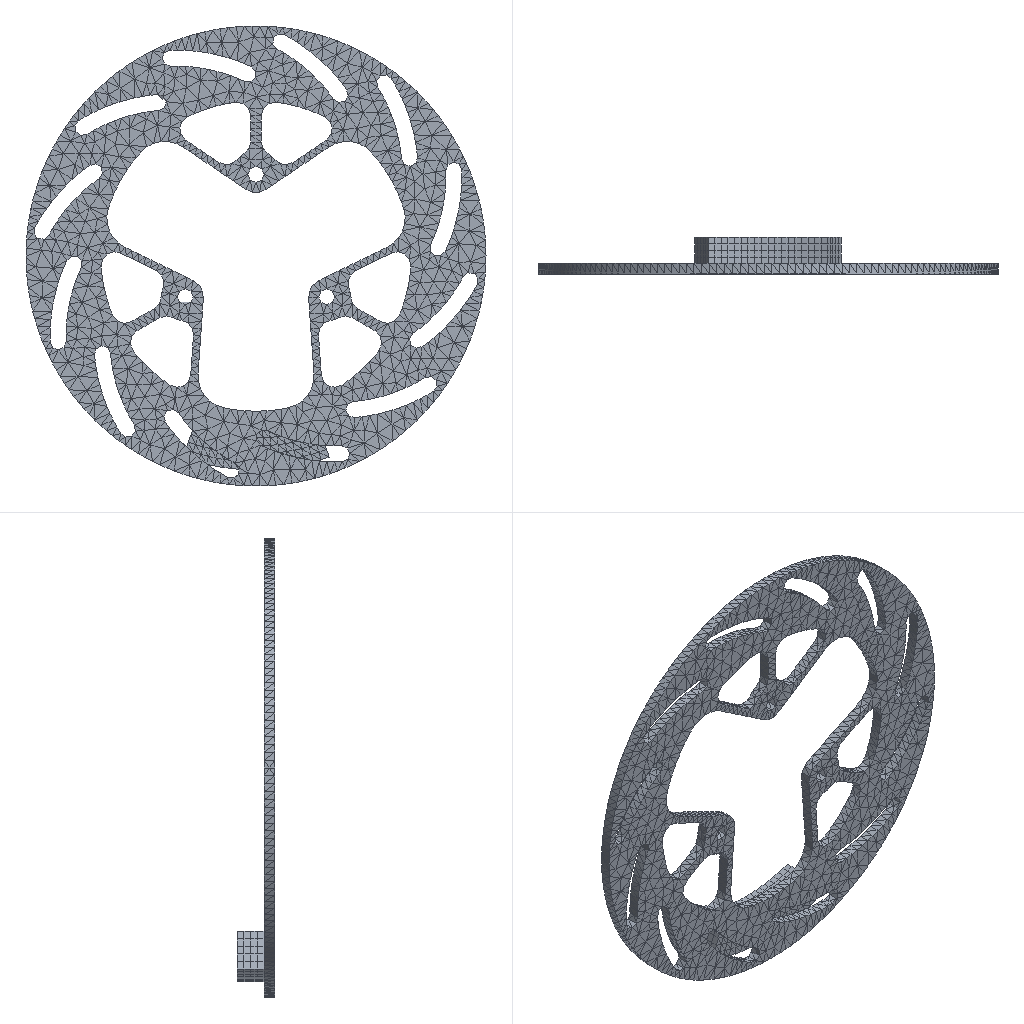Simulation study | ansys workbench
Set-up summary:
category,name,step,type,value,unit,region
solver,ansys_workbench
units,mm-N-s-tonne (MPa),,stated,"/units,MPA"
analysis,LS1,,transient thermal
load_step,LS1,LS1,transient thermal,nsubst=100; time=5
mesh,nodes,,,16602
mesh,elements,,,11231
element_type,SOLID291,,,6582
element_type,SURF152,,,3759
element_type,SOLID279,,,360
element_type,TARGE170,,,265
element_type,CONTA174,,,265
material,HT250,,E,120000,tonne s^-2 mm^-1
material,HT250,,nu,0.26
material,HT250,,density,7.2e-09,tonne mm^-3
material,HT250,,conductivity,44.3,tonne mm s^-3 C^-1
material,HT250,,specific_heat,4.5e+08,mm^2 s^-2 C^-1
material,HT250,,cte,6e-06,C^-1
load,Define Uniform Initial temperature,model,body load temp,22,,all
load,"Create ""?""",LS1,heat flux,1800,,SURF152 #5
load,"Create ""? 2""",LS1,heat flux,1800,,SURF152 #6
load,"Create ""______""",LS1,convection,0.1,,SURF152 #7
contact,Contact Region,,bonded (always),element=CONTA174
Ansys APDL input file, long lists of numbers shortened:
/batch
/config,noeldb,1     ! force off writing results to database
*get,_wallstrt,active,,time,wall
! ANSYS input file written by Workbench version 2021 R1
! File used for geometry attach:
/title,_______--___ (B5)
! ****** Begin Custom Load Command Snippet ******
/COM, ACT Extensions:
/COM,     LSDYNA, 2021.1
/COM,
! ****** End   Custom Load Command Snippet ******
*DIM,_wb_ProjectScratch_dir,string,248
_wb_ProjectScratch_dir(1) = ''
*DIM,_wb_SolverFiles_dir,string,248
_wb_SolverFiles_dir(1) = ''
*DIM,_wb_userfiles_dir,string,248
_wb_userfiles_dir(1) = ''
/com,--- Data in consistent NMM units. See Solving Units in the help system for more information.
/units,MPA
/nopr
/wb,file,start              !  signify a WB generated input file
/prep7
! Turn off shape checking because checks already performed inside WB mesher.
! See help system for more information.
SHPP,OFF,,NOWARN
/nolist
etcon,set             ! allow ANSYS to choose best KEYOP's for 180x elements, resets any applicable keyopt to MAPDL defaults
/com,*********** Nodes for the whole assembly ***********
nblock,3,,18262
(1i9,3e20.9e3)
        1     2.076216784E+01     6.500000000E+00    -6.475285620E+01
! (16601 more lines like these left out)
-1
/wb,elem,start            !  set before creation of elements
/com,*********** Elements for Body 1 "______|______1" ***********
et,1,291
eblock,19,solid,,6582
(19i9)
        1        1        1        1        0        0        0        0       10        0      361     2164     4762     4635     2876     5525    16570     5524     5520
! (13163 more lines like these left out)
-1
/com,*********** Elements for Body 2 "______-0|____-____1" ***********
et,2,279
eblock,19,solid,,360
(19i9)
        2        2        2        2        0        0        0        0       20        0        1        1      466      460      387      272      475      456      455
! (719 more lines like these left out)
-1
/wb,elem,end               !  done creating elements
/com,*********** Send User Defined Coordinate System(s) ***********
csys,0
toffst,273.15,  ! Temperature offset from absolute zero
/wb,mat,start              !  starting to send materials
/com,*********** Send Materials ***********
MP,DENS,1,7.2e-09,	! tonne mm^-3
MP,ALPX,1,6e-06,	! C^-1
MP,EX,1,120000,	! tonne s^-2 mm^-1
MP,NUXY,1,0.26,
MP,KXX,1,44.3,	! tonne mm s^-3 C^-1
MP,C,1,450000000,	! mm^2 s^-2 C^-1
MP,DENS,2,7.2e-09,	! tonne mm^-3
MP,ALPX,2,6e-06,	! C^-1
MP,EX,2,120000,	! tonne s^-2 mm^-1
MP,NUXY,2,0.26,
MP,KXX,2,44.3,	! tonne mm s^-3 C^-1
MP,C,2,450000000,	! mm^2 s^-2 C^-1
/wb,mat,end                !  done sending materials
!************************* Model Summary ********************
!______|______1,	HT250,	matid,	1
!______-0|____-____1,	HT250,	matid,	2
!************************* End Model Summary ********************
! get the diagonal of the bounding box. Needed later for other things
*get,_xmin,node,,mnloc,x
*get,_ymin,node,,mnloc,y
*get,_zmin,node,,mnloc,z
*get,_xmax,node,,mxloc,x
*get,_ymax,node,,mxloc,y
*get,_zmax,node,,mxloc,z
_ASMDIAG=(_xmax-_xmin)*(_xmax-_xmin)+(_ymax-_ymin)*(_ymax-_ymin)+(_zmax-_zmin)*(_zmax-_zmin)
_ASMDIAG=SQRT(_ASMDIAG)
/wb,contact,start          !  starting to send contact
/com,*********** Create Contact "接触区域" ***********
/com,            Real Constant Set For Above Contact Is 4 & 3
*set,tid,4
*set,cid,3
r,tid
r,cid
et,tid,170
et,cid,174
eblock,10,,,175
(15i9)
    12335        4        4        4        0     2393     2394     2894     2894     6917     6925     2894     6918
! (174 more lines like these left out)
-1
eblock,10,,,175
(15i9)
    12510        3        3        3        0     2393     2394     2894     2894     6917     6925     2894     6918
! (174 more lines like these left out)
-1
eblock,10,,,90
(15i9)
    12685        3        4        3        0      455      272      475      456     1469     1470     1846     1844
! (89 more lines like these left out)
-1
eblock,10,,,90
(15i9)
    12775        4        3        4        0      455      272      475      456     1469     1470     1846     1844
! (89 more lines like these left out)
-1
keyo,cid,8,2               ! auto create asymmetric contact (from Program Controlled setting)
keyo,cid,10,0              ! adjust contact stiffness each NR iteration (from Program Controlled setting)
keyo,cid,12,5              ! bonded always
keyo,cid,18,1              ! small sliding turned on by application
keyo,cid,2,0               ! augmented Lagrange (from Program Controlled setting)
keyo,cid,4,0               ! on Gauss point (from Program Controlled setting)
keyo,cid,9,1               ! ignore initial gaps/penetration
keyo,cid,7,0               ! No Prediction
rmod,tid,3,10.      ! FKN
rmod,tid,5,0.       ! ICONT
rmod,tid,6,0.       ! PINB
rmod,tid,10,0.      ! CNOF
rmod,tid,12,0.      ! FKT
rmod,tid,36,52      ! WB DSID
rmod,cid,3,10.      ! FKN
rmod,cid,5,0.       ! ICONT
rmod,cid,6,0.       ! PINB
rmod,cid,10,0.      ! CNOF
rmod,cid,12,0.      ! FKT
rmod,cid,36,52      ! WB DSID
*set,_maxkxx,443000.
rmod,cid,14,_maxkxx/_ASMDIAG         ! TCC, Divide by Length since Traction Based
rmod,tid,14,_maxkxx/_ASMDIAG      ! TCC, Divide by Length since Traction Based
keyo,cid,1,2     ! Pure thermal contact
nsel,all
esel,all
/wb,contact,end            !  done creating contacts
/golist
/wb,load,start             !  starting to send loads
/com,*********** Create "热通量" ***********
et,5,152
eblock,10,,,88
(15i9)
    12865        5        5        5        0     2893     3952     2941     2941     9727     9996     2941     9726
! (87 more lines like these left out)
-1
esel,s,type,,5
keyop,5,8,1      ! include heat flux
*DIM,_loadvari36,TABLE,2,1,1,TIME,
! Time values
_loadvari36(1,0,1) = 0.
_loadvari36(2,0,1) = 5.
! Load values
_loadvari36(1,1,1) = 0.
_loadvari36(2,1,1) = 1800.
/com,*********** Create "热通量 2" ***********
et,6,152
eblock,10,,,90
(15i9)
    12953        6        6        6        0      455      272      475      456     1469     1470     1846     1844
! (89 more lines like these left out)
-1
esel,s,type,,6
keyop,6,8,1      ! include heat flux
*DIM,_loadvari56,TABLE,2,1,1,TIME,
! Time values
_loadvari56(1,0,1) = 0.
_loadvari56(2,0,1) = 5.
! Load values
_loadvari56(1,1,1) = 0.
_loadvari56(2,1,1) = 1800.
esel,all
fcum,add                   ! add nodal forces up (needed in case have loads on the same edge,vertex)
fcum                       ! reset default on fcum command since done sending WB F loads
/com,*********** Create "______" ***********
et,7,152
eblock,10,,,3581
(15i9)
    13043        7        7        7        0     2957     3725     2958     2958    10068    10071     2958    10066
! (3580 more lines like these left out)
-1
esel,s,type,,7
keyop,7,8,2.
keyop,7,13,0
*DIM,_convvari38,TABLE,2,1,1,TIME,
! Time values
_convvari38(1,0,1) = 0.
_convvari38(2,0,1) = 5.
! Load values
_convvari38(1,1,1) = 0.1
_convvari38(2,1,1) = 0.1
esel,all
/com,***************** Define Uniform Initial temperature ***************
tunif,22.
/gst,on,on
fini
*get,_numnode,node,0,count
*get,_numelem,elem,0,count
*get, _MAXELEMNUM, elem, 0, NUM, MAX
*get, _MAXNODENUM, node, 0, NUM, MAX
*get, _MAXELEMTYPE, etyp, 0, NUM, MAX
*get, _MAXREALCONST, real, 0, NUM, MAX
/go
/wb,load,end               !  done creating loads
/com,--- Number of total nodes = %_numnode%
/com,--- Number of contact elements = 4289
/com,--- Number of spring elements = 0
/com,--- Number of bearing elements = 0
/com,--- Number of solid elements = 6942
/com,--- Number of condensed parts = 0
/com,--- Number of total elements = %_numelem%
*get,_wallbsol,active,,time,wall
/com,****************************************************************************
/com,*************************    SOLUTION       ********************************
/com,****************************************************************************
/solu
antype,4                   ! transient analysis
kbc,1                      ! stepped BC's
!eqsl,sparse               ! using sparse solver which is default so no eqsl command needed
cntr,print,1               ! print out contact info and also make no initial contact an error
rescontrol,,none                 ! Do not keep any restart files
dmpoption,emat,no             ! Don't combine emat file for DANSYS
dmpoption,esav,no             ! Don't combine esav file for DANSYS
thopt,quasi,5.e-002
nlhist,nsol,MAX_TEMP,temp,max
nlhist,nsol,MIN_TEMP,temp,min
/com,********* Initial Time Increment Check And Fourier Modulus *********
/com, Specified Initial Time Increment: 0.05
/com, Estimated Increment Needed, le*le/alpha, Body 1: 0.2709
/com, Estimated Increment Needed, le*le/alpha, Body 2: 0.5583
/com,****************************************************
/com,******************* SOLVE FOR LS 1 OF 1 ****************
esel,s,type,,5
nsle
sf,all,hflux,%_loadvari36%
esel,s,type,,6
nsle
sf,all,hflux,%_loadvari56%
nsel,all
esel,all
esel,s,type,,7
nsle
sf,all,conv,%_convvari38%,22.
nsel,all
esel,all
autots,on
nsub,100,1000,10
time,5.
timint,on                  ! Turn on time integration effects
outres,erase
outres,all,none
outres,nsol,all
outres,rsol,all
outres,eangl,all
outres,veng,all
outres,fflux,all
outres,cont,all
/nopr
esel,s,type,,7
cm,_elmisc,elem
esel,all
/gopr
outres,misc,all,_elmisc
cnvtol,heat,,.001,,1.e-003    ! Program Controlled. Set MINREF equivalent of 1e-6 Watts
! *********** WB SOLVE COMMAND ***********
! check interactive state
*get,ANSINTER_,active,,int
*if,ANSINTER_,ne,0,then
/eof
*endif
solve
/com *************** Write FE CONNECTORS *********
CEWRITE,file,ce,,INTE
/com,****************************************************
/com,*************** FINISHED SOLVE FOR LS 1 *************
*get,_wallasol,active,,time,wall
/post1
xmlo,ENCODING,ISO-8859-1
xmlo,parm
/xml,parm,xml
fini
/gopr
*get,_walldone,active,,time,wall
_preptime=(_wallbsol-_wallstrt)*3600
_solvtime=(_wallasol-_wallbsol)*3600
_posttime=(_walldone-_wallasol)*3600
_totaltim=(_walldone-_wallstrt)*3600
*get,_dlbratio,active,0,solu,dlbr
*get,_combtime,active,0,solu,comb
/com,--- Total number of nodes = %_numnode%
/com,--- Total number of elements = %_numelem%
/com,--- Element load balance ratio = %_dlbratio%
/com,--- Time to combine distributed files = %_combtime%
/wb,file,end               ! done with WB generated input
Results summary:
result,analyses[0].index,,,1
result,analyses[0].system,,,SYS-1
result,analyses[0].deck,,,deck.dat
result,analyses[0].solve_status,,,completed
result,analyses[0].analysis_type,,,static
result,analyses[0].physics,,,thermal
result,analyses[0].unit_system,,,"NMM: mm, ton, N, s, mV, mA, degC"
result,analyses[0].n_sets,,,17
result,analyses[0].load_steps[0].set,set=17,,17
result,analyses[0].load_steps[0].time_or_freq,set=17,,5
result,analyses[0].load_steps[0].max_temperature,set=17,,327.177
result,analyses[0].load_steps[0].min_temperature,set=17,,22
result,geometry_export[0][0],,,.step
result,geometry_export[0][1],,,ok
result,geometry_export[0][2],,,2